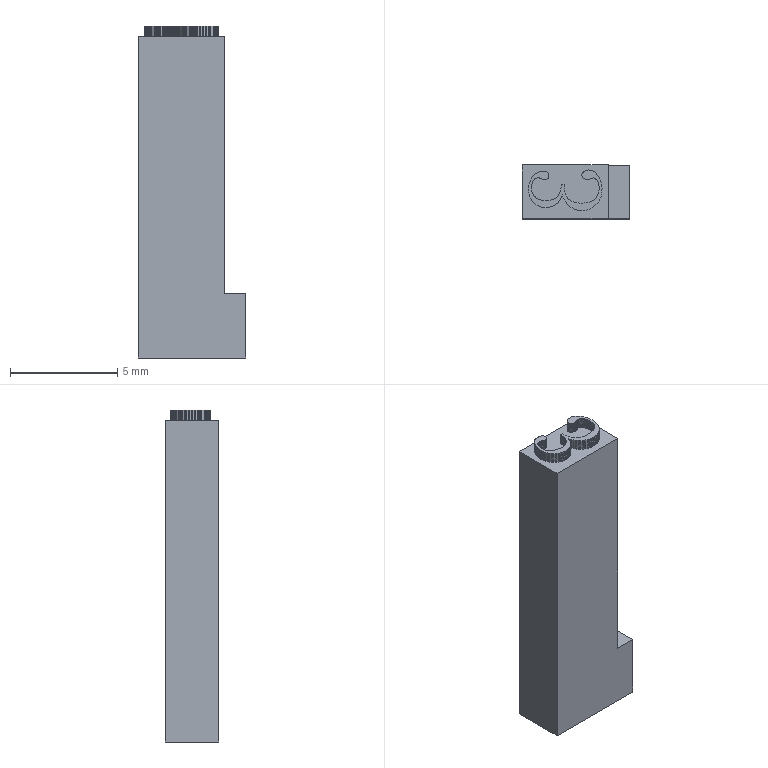Part | NX | features DIE-28 2 | 1 solid | 307 faces | box 5 x 2.5 x 15.5 mm | volume 158.404 mm3 | plane 307